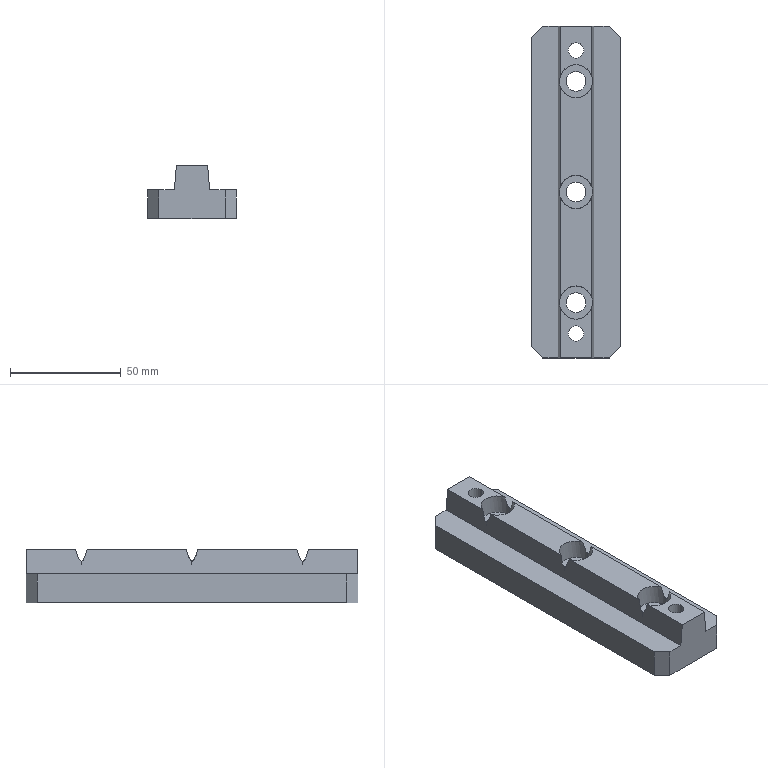Part | Creo | 1 solid | 36 faces | box 40 x 150 x 24 mm | volume 92701 mm3 | plane 20 | cylinder 16 | commonest cylinder face diameters 9 x6 15 x6 7 x4